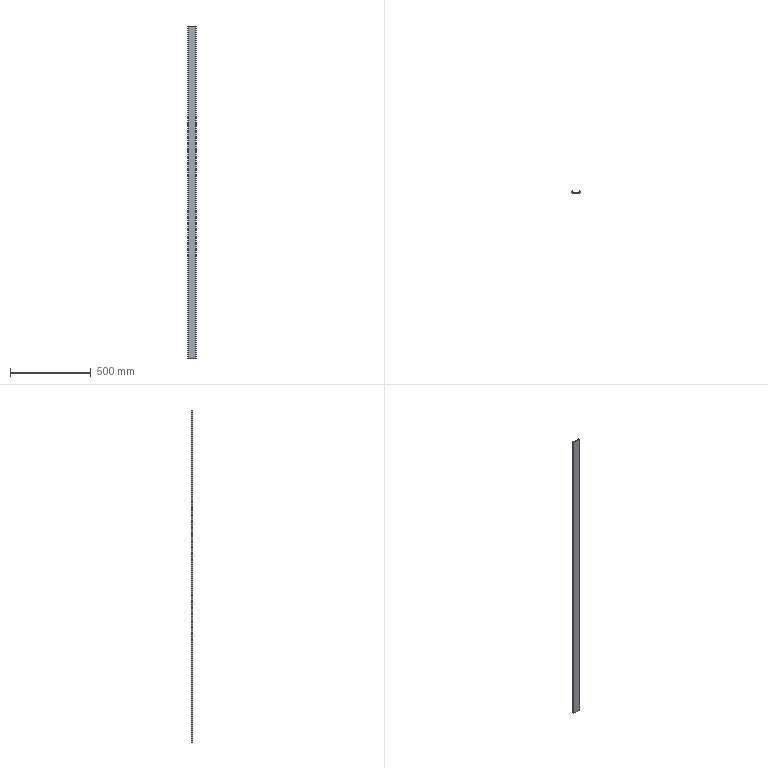Part | STEP file | 31E-01030QY25 | 1 solid | 32 faces | box 50 x 9.195 x 2050 mm | volume 179814 mm3 | cylinder 16 | plane 16 | commonest cylinder face diameters 1 x8 1.2 x6 2 x2
STEP:
#1=CARTESIAN_POINT('',(0.2485,8.595,1025.));
#2=VERTEX_POINT('',#1);
#3=CARTESIAN_POINT('',(0.4243,8.171,1025.));
#4=VERTEX_POINT('',#3);
#5=CARTESIAN_POINT('',(0.8485,8.595,1025.));
#6=DIRECTION('',(0.,0.,-1.));
#7=AXIS2_PLACEMENT_3D('',#5,#6,$);
#8=CIRCLE('',#7,0.6);
#9=EDGE_CURVE('',#2,#4,#8,.F.);
#10=ORIENTED_EDGE('',*,*,#9,.F.);
#11=CARTESIAN_POINT('',(0.2485,8.595,-1025.));
#12=VERTEX_POINT('',#11);
#13=CARTESIAN_POINT('',(0.2485,8.595,1025.));
#14=DIRECTION('',(0.,0.,-1.));
#15=VECTOR('',#14,1.);
#16=LINE('',#13,#15);
#17=EDGE_CURVE('',#2,#12,#16,.T.);
#18=ORIENTED_EDGE('',*,*,#17,.T.);
#19=CARTESIAN_POINT('',(0.4243,8.171,-1025.));
#20=VERTEX_POINT('',#19);
#21=CARTESIAN_POINT('',(0.8485,8.595,-1025.));
#22=DIRECTION('',(0.,0.,-1.));
#23=AXIS2_PLACEMENT_3D('',#21,#22,$);
#24=CIRCLE('',#23,0.6);
#25=EDGE_CURVE('',#20,#12,#24,.T.);
#26=ORIENTED_EDGE('',*,*,#25,.F.);
#27=CARTESIAN_POINT('',(0.4243,8.171,1025.));
#28=DIRECTION('',(0.,0.,-1.));
#29=VECTOR('',#28,1.);
#30=LINE('',#27,#29);
#31=EDGE_CURVE('',#4,#20,#30,.T.);
#32=ORIENTED_EDGE('',*,*,#31,.F.);
#33=EDGE_LOOP('',(#10,#18,#26,#32));
#34=FACE_OUTER_BOUND('',#33,.T.);
#35=CARTESIAN_POINT('',(0.8485,8.595,1025.));
#36=DIRECTION('',(0.,0.,-1.));
#37=DIRECTION('',(1.,0.,0.));
#38=AXIS2_PLACEMENT_3D('',#35,#36,#37);
#39=CYLINDRICAL_SURFACE('',#38,0.6);
#40=ADVANCED_FACE('',(#34),#39,.T.);
#41=CARTESIAN_POINT('',(1.273,9.019,1025.));
#42=VERTEX_POINT('',#41);
#43=CARTESIAN_POINT('',(0.4243,9.019,1025.));
#44=VERTEX_POINT('',#43);
#45=CARTESIAN_POINT('',(1.273,9.019,1025.));
#46=CARTESIAN_POINT('',(1.219,9.073,1025.));
#47=CARTESIAN_POINT('',(1.158,9.118,1025.));
#48=CARTESIAN_POINT('',(1.089,9.152,1025.));
#49=CARTESIAN_POINT('',(0.9442,9.199,1025.));
#50=CARTESIAN_POINT('',(0.7916,9.2,1025.));
#51=CARTESIAN_POINT('',(0.7159,9.188,1025.));
#52=CARTESIAN_POINT('',(0.6071,9.152,1025.));
#53=CARTESIAN_POINT('',(0.5104,9.093,1025.));
#54=CARTESIAN_POINT('',(0.4796,9.07,1025.));
#55=CARTESIAN_POINT('',(0.4509,9.046,1025.));
#56=CARTESIAN_POINT('',(0.4243,9.019,1025.));
#57=B_SPLINE_CURVE_WITH_KNOTS('',5,(#45,#46,#47,#48,#49,#50,#51,#52,#53,#54,#55,#56),.UNSPECIFIED.,.F.,.U.,(6,3,3,6),(0.,0.5331,1.066,1.332),.UNSPECIFIED.);
#58=EDGE_CURVE('',#42,#44,#57,.T.);
#59=ORIENTED_EDGE('',*,*,#58,.T.);
#60=CARTESIAN_POINT('',(0.4243,9.019,1025.));
#61=CARTESIAN_POINT('',(0.3843,8.979,1025.));
#62=CARTESIAN_POINT('',(0.349,8.935,1025.));
#63=CARTESIAN_POINT('',(0.3192,8.886,1025.));
#64=CARTESIAN_POINT('',(0.2795,8.8,1025.));
#65=CARTESIAN_POINT('',(0.2574,8.708,1025.));
#66=CARTESIAN_POINT('',(0.2515,8.67,1025.));
#67=CARTESIAN_POINT('',(0.2485,8.633,1025.));
#68=CARTESIAN_POINT('',(0.2485,8.595,1025.));
#69=B_SPLINE_CURVE_WITH_KNOTS('',5,(#60,#61,#62,#63,#64,#65,#66,#67,#68),.UNSPECIFIED.,.F.,.U.,(6,3,6),(0.,0.3999,0.6659),.UNSPECIFIED.);
#70=EDGE_CURVE('',#44,#2,#69,.T.);
#71=ORIENTED_EDGE('',*,*,#70,.T.);
#72=ORIENTED_EDGE('',*,*,#9,.T.);
#73=CARTESIAN_POINT('',(2.898,5.697,1025.));
#74=VERTEX_POINT('',#73);
#75=CARTESIAN_POINT('',(1.661,6.934,1025.));
#76=DIRECTION('',(0.7071,-0.7071,0.));
#77=VECTOR('',#76,1.);
#78=LINE('',#75,#77);
#79=EDGE_CURVE('',#4,#74,#78,.T.);
#80=ORIENTED_EDGE('',*,*,#79,.T.);
#81=CARTESIAN_POINT('',(0.3706,5.02,1025.));
#82=VERTEX_POINT('',#81);
#83=CARTESIAN_POINT('',(1.634,5.359,1025.));
#84=DIRECTION('',(-0.9659,-0.2588,0.));
#85=VECTOR('',#84,1.);
#86=LINE('',#83,#85);
#87=EDGE_CURVE('',#74,#82,#86,.T.);
#88=ORIENTED_EDGE('',*,*,#87,.T.);
#89=CARTESIAN_POINT('',(0.,4.537,1025.));
#90=VERTEX_POINT('',#89);
#91=CARTESIAN_POINT('',(0.3706,5.02,1025.));
#92=CARTESIAN_POINT('',(0.32,5.007,1025.));
#93=CARTESIAN_POINT('',(0.2712,4.986,1025.));
#94=CARTESIAN_POINT('',(0.2253,4.96,1025.));
#95=CARTESIAN_POINT('',(0.1416,4.896,1025.));
#96=CARTESIAN_POINT('',(0.07725,4.812,1025.));
#97=CARTESIAN_POINT('',(0.05076,4.766,1025.));
#98=CARTESIAN_POINT('',(0.02052,4.693,1025.));
#99=CARTESIAN_POINT('',(0.005155,4.616,1025.));
#100=CARTESIAN_POINT('',(0.001709,4.589,1025.));
#101=CARTESIAN_POINT('',(0.,4.563,1025.));
#102=CARTESIAN_POINT('',(0.,4.537,1025.));
#103=B_SPLINE_CURVE_WITH_KNOTS('',5,(#91,#92,#93,#94,#95,#96,#97,#98,#99,#100,#101,#102),.UNSPECIFIED.,.F.,.U.,(6,3,3,6),(0.,0.3702,0.7405,0.9253),.UNSPECIFIED.);
#104=EDGE_CURVE('',#82,#90,#103,.T.);
#105=ORIENTED_EDGE('',*,*,#104,.T.);
#106=CARTESIAN_POINT('',(0.,1.,1025.));
#107=VERTEX_POINT('',#106);
#108=CARTESIAN_POINT('',(0.,2.769,1025.));
#109=DIRECTION('',(0.,-1.,0.));
#110=VECTOR('',#109,1.);
#111=LINE('',#108,#110);
#112=EDGE_CURVE('',#90,#107,#111,.T.);
#113=ORIENTED_EDGE('',*,*,#112,.T.);
#114=CARTESIAN_POINT('',(1.,0.,1025.));
#115=VERTEX_POINT('',#114);
#116=CARTESIAN_POINT('',(0.,1.,1025.));
#117=CARTESIAN_POINT('',(0.,0.902,1025.));
#118=CARTESIAN_POINT('',(0.012,0.804,1025.));
#119=CARTESIAN_POINT('',(0.036,0.708,1025.));
#120=CARTESIAN_POINT('',(0.107,0.5238,1025.));
#121=CARTESIAN_POINT('',(0.2204,0.3622,1025.));
#122=CARTESIAN_POINT('',(0.2868,0.2888,1025.));
#123=CARTESIAN_POINT('',(0.4361,0.1597,1025.));
#124=CARTESIAN_POINT('',(0.6122,0.0704,1025.));
#125=CARTESIAN_POINT('',(0.7053,0.03682,1025.));
#126=CARTESIAN_POINT('',(0.8215,0.01049,1025.));
#127=CARTESIAN_POINT('',(0.9393,0.001534,1025.));
#128=CARTESIAN_POINT('',(0.9596,0.0005109,1025.));
#129=CARTESIAN_POINT('',(0.9798,0.000000001,1025.));
#130=CARTESIAN_POINT('',(1.,0.000000001,1025.));
#131=B_SPLINE_CURVE_WITH_KNOTS('',5,(#116,#117,#118,#119,#120,#121,#122,#123,#124,#125,#126,#127,#128,#129,#130),.UNSPECIFIED.,.F.,.U.,(6,3,3,3,6),(0.,0.6928,1.386,2.078,2.221),.UNSPECIFIED.);
#132=EDGE_CURVE('',#107,#115,#131,.T.);
#133=ORIENTED_EDGE('',*,*,#132,.T.);
#134=CARTESIAN_POINT('',(49.,0.,1025.));
#135=VERTEX_POINT('',#134);
#136=CARTESIAN_POINT('',(25.,0.000000001,1025.));
#137=DIRECTION('',(1.,0.,0.));
#138=VECTOR('',#137,1.);
#139=LINE('',#136,#138);
#140=EDGE_CURVE('',#115,#135,#139,.T.);
#141=ORIENTED_EDGE('',*,*,#140,.T.);
#142=CARTESIAN_POINT('',(50.,1.,1025.));
#143=VERTEX_POINT('',#142);
#144=CARTESIAN_POINT('',(49.,0.000000001,1025.));
#145=CARTESIAN_POINT('',(49.098,0.000000001,1025.));
#146=CARTESIAN_POINT('',(49.196,0.012,1025.));
#147=CARTESIAN_POINT('',(49.292,0.036,1025.));
#148=CARTESIAN_POINT('',(49.476,0.107,1025.));
#149=CARTESIAN_POINT('',(49.638,0.2204,1025.));
#150=CARTESIAN_POINT('',(49.711,0.2868,1025.));
#151=CARTESIAN_POINT('',(49.84,0.4361,1025.));
#152=CARTESIAN_POINT('',(49.93,0.6122,1025.));
#153=CARTESIAN_POINT('',(49.963,0.7053,1025.));
#154=CARTESIAN_POINT('',(49.99,0.8215,1025.));
#155=CARTESIAN_POINT('',(49.998,0.9393,1025.));
#156=CARTESIAN_POINT('',(49.999,0.9596,1025.));
#157=CARTESIAN_POINT('',(50.,0.9798,1025.));
#158=CARTESIAN_POINT('',(50.,1.,1025.));
#159=B_SPLINE_CURVE_WITH_KNOTS('',5,(#144,#145,#146,#147,#148,#149,#150,#151,#152,#153,#154,#155,#156,#157,#158),.UNSPECIFIED.,.F.,.U.,(6,3,3,3,6),(0.,0.6928,1.386,2.078,2.221),.UNSPECIFIED.);
#160=EDGE_CURVE('',#135,#143,#159,.T.);
#161=ORIENTED_EDGE('',*,*,#160,.T.);
#162=CARTESIAN_POINT('',(50.,4.537,1025.));
#163=VERTEX_POINT('',#162);
#164=CARTESIAN_POINT('',(50.,2.769,1025.));
#165=DIRECTION('',(0.,1.,0.));
#166=VECTOR('',#165,1.);
#167=LINE('',#164,#166);
#168=EDGE_CURVE('',#143,#163,#167,.T.);
#169=ORIENTED_EDGE('',*,*,#168,.T.);
#170=CARTESIAN_POINT('',(49.629,5.02,1025.));
#171=VERTEX_POINT('',#170);
#172=CARTESIAN_POINT('',(50.,4.537,1025.));
#173=CARTESIAN_POINT('',(50.,4.589,1025.));
#174=CARTESIAN_POINT('',(49.993,4.642,1025.));
#175=CARTESIAN_POINT('',(49.979,4.693,1025.));
#176=CARTESIAN_POINT('',(49.939,4.791,1025.));
#177=CARTESIAN_POINT('',(49.875,4.874,1025.));
#178=CARTESIAN_POINT('',(49.837,4.912,1025.));
#179=CARTESIAN_POINT('',(49.774,4.96,1025.));
#180=CARTESIAN_POINT('',(49.704,4.995,1025.));
#181=CARTESIAN_POINT('',(49.679,5.005,1025.));
#182=CARTESIAN_POINT('',(49.655,5.013,1025.));
#183=CARTESIAN_POINT('',(49.629,5.02,1025.));
#184=B_SPLINE_CURVE_WITH_KNOTS('',5,(#172,#173,#174,#175,#176,#177,#178,#179,#180,#181,#182,#183),.UNSPECIFIED.,.F.,.U.,(6,3,3,6),(0.,0.3702,0.7405,0.9253),.UNSPECIFIED.);
#185=EDGE_CURVE('',#163,#171,#184,.T.);
#186=ORIENTED_EDGE('',*,*,#185,.T.);
#187=CARTESIAN_POINT('',(47.102,5.697,1025.));
#188=VERTEX_POINT('',#187);
#189=CARTESIAN_POINT('',(48.366,5.359,1025.));
#190=DIRECTION('',(-0.9659,0.2588,0.));
#191=VECTOR('',#190,1.);
#192=LINE('',#189,#191);
#193=EDGE_CURVE('',#171,#188,#192,.T.);
#194=ORIENTED_EDGE('',*,*,#193,.T.);
#195=CARTESIAN_POINT('',(49.576,8.171,1025.));
#196=VERTEX_POINT('',#195);
#197=CARTESIAN_POINT('',(48.339,6.934,1025.));
#198=DIRECTION('',(0.7071,0.7071,0.));
#199=VECTOR('',#198,1.);
#200=LINE('',#197,#199);
#201=EDGE_CURVE('',#188,#196,#200,.T.);
#202=ORIENTED_EDGE('',*,*,#201,.T.);
#203=CARTESIAN_POINT('',(49.751,8.595,1025.));
#204=VERTEX_POINT('',#203);
#205=CARTESIAN_POINT('',(49.576,8.171,1025.));
#206=CARTESIAN_POINT('',(49.629,8.224,1025.));
#207=CARTESIAN_POINT('',(49.674,8.286,1025.));
#208=CARTESIAN_POINT('',(49.709,8.354,1025.));
#209=CARTESIAN_POINT('',(49.738,8.445,1025.));
#210=CARTESIAN_POINT('',(49.749,8.539,1025.));
#211=CARTESIAN_POINT('',(49.751,8.557,1025.));
#212=CARTESIAN_POINT('',(49.751,8.576,1025.));
#213=CARTESIAN_POINT('',(49.751,8.595,1025.));
#214=B_SPLINE_CURVE_WITH_KNOTS('',5,(#205,#206,#207,#208,#209,#210,#211,#212,#213),.UNSPECIFIED.,.F.,.U.,(6,3,6),(0.,0.5331,0.6664),.UNSPECIFIED.);
#215=EDGE_CURVE('',#196,#204,#214,.T.);
#216=ORIENTED_EDGE('',*,*,#215,.T.);
#217=CARTESIAN_POINT('',(49.576,9.019,1025.));
#218=VERTEX_POINT('',#217);
#219=CARTESIAN_POINT('',(49.751,8.595,1025.));
#220=CARTESIAN_POINT('',(49.751,8.652,1025.));
#221=CARTESIAN_POINT('',(49.745,8.708,1025.));
#222=CARTESIAN_POINT('',(49.731,8.764,1025.));
#223=CARTESIAN_POINT('',(49.699,8.853,1025.));
#224=CARTESIAN_POINT('',(49.649,8.933,1025.));
#225=CARTESIAN_POINT('',(49.627,8.964,1025.));
#226=CARTESIAN_POINT('',(49.602,8.993,1025.));
#227=CARTESIAN_POINT('',(49.576,9.019,1025.));
#228=B_SPLINE_CURVE_WITH_KNOTS('',5,(#219,#220,#221,#222,#223,#224,#225,#226,#227),.UNSPECIFIED.,.F.,.U.,(6,3,6),(0.6664,1.066,1.332),.UNSPECIFIED.);
#229=EDGE_CURVE('',#204,#218,#228,.T.);
#230=ORIENTED_EDGE('',*,*,#229,.T.);
#231=CARTESIAN_POINT('',(48.727,9.019,1025.));
#232=VERTEX_POINT('',#231);
#233=CARTESIAN_POINT('',(49.576,9.019,1025.));
#234=CARTESIAN_POINT('',(49.522,9.073,1025.));
#235=CARTESIAN_POINT('',(49.461,9.118,1025.));
#236=CARTESIAN_POINT('',(49.392,9.152,1025.));
#237=CARTESIAN_POINT('',(49.247,9.199,1025.));
#238=CARTESIAN_POINT('',(49.095,9.2,1025.));
#239=CARTESIAN_POINT('',(49.019,9.188,1025.));
#240=CARTESIAN_POINT('',(48.91,9.152,1025.));
#241=CARTESIAN_POINT('',(48.813,9.093,1025.));
#242=CARTESIAN_POINT('',(48.782,9.07,1025.));
#243=CARTESIAN_POINT('',(48.754,9.046,1025.));
#244=CARTESIAN_POINT('',(48.727,9.019,1025.));
#245=B_SPLINE_CURVE_WITH_KNOTS('',5,(#233,#234,#235,#236,#237,#238,#239,#240,#241,#242,#243,#244),.UNSPECIFIED.,.F.,.U.,(6,3,3,6),(0.,0.5331,1.066,1.332),.UNSPECIFIED.);
#246=EDGE_CURVE('',#218,#232,#245,.T.);
#247=ORIENTED_EDGE('',*,*,#246,.T.);
#248=CARTESIAN_POINT('',(45.396,5.688,1025.));
#249=VERTEX_POINT('',#248);
#250=CARTESIAN_POINT('',(47.062,7.354,1025.));
#251=DIRECTION('',(-0.7071,-0.7071,0.));
#252=VECTOR('',#251,1.);
#253=LINE('',#250,#252);
#254=EDGE_CURVE('',#232,#249,#253,.T.);
#255=ORIENTED_EDGE('',*,*,#254,.T.);
#256=CARTESIAN_POINT('',(45.25,5.335,1025.));
#257=VERTEX_POINT('',#256);
#258=CARTESIAN_POINT('',(45.396,5.688,1025.));
#259=CARTESIAN_POINT('',(45.363,5.655,1025.));
#260=CARTESIAN_POINT('',(45.334,5.618,1025.));
#261=CARTESIAN_POINT('',(45.309,5.577,1025.));
#262=CARTESIAN_POINT('',(45.276,5.506,1025.));
#263=CARTESIAN_POINT('',(45.257,5.429,1025.));
#264=CARTESIAN_POINT('',(45.252,5.398,1025.));
#265=CARTESIAN_POINT('',(45.25,5.366,1025.));
#266=CARTESIAN_POINT('',(45.25,5.335,1025.));
#267=B_SPLINE_CURVE_WITH_KNOTS('',5,(#258,#259,#260,#261,#262,#263,#264,#265,#266),.UNSPECIFIED.,.F.,.U.,(6,3,6),(0.,0.3332,0.5549),.UNSPECIFIED.);
#268=EDGE_CURVE('',#249,#257,#267,.T.);
#269=ORIENTED_EDGE('',*,*,#268,.T.);
#270=CARTESIAN_POINT('',(45.621,4.852,1025.));
#271=VERTEX_POINT('',#270);
#272=CARTESIAN_POINT('',(45.25,5.335,1025.));
#273=CARTESIAN_POINT('',(45.25,5.283,1025.));
#274=CARTESIAN_POINT('',(45.257,5.23,1025.));
#275=CARTESIAN_POINT('',(45.27,5.179,1025.));
#276=CARTESIAN_POINT('',(45.311,5.081,1025.));
#277=CARTESIAN_POINT('',(45.375,4.998,1025.));
#278=CARTESIAN_POINT('',(45.413,4.96,1025.));
#279=CARTESIAN_POINT('',(45.476,4.912,1025.));
#280=CARTESIAN_POINT('',(45.546,4.877,1025.));
#281=CARTESIAN_POINT('',(45.57,4.867,1025.));
#282=CARTESIAN_POINT('',(45.595,4.859,1025.));
#283=CARTESIAN_POINT('',(45.621,4.852,1025.));
#284=B_SPLINE_CURVE_WITH_KNOTS('',5,(#272,#273,#274,#275,#276,#277,#278,#279,#280,#281,#282,#283),.UNSPECIFIED.,.F.,.U.,(6,3,3,6),(0.,0.3702,0.7405,0.9253),.UNSPECIFIED.);
#285=EDGE_CURVE('',#257,#271,#284,.T.);
#286=ORIENTED_EDGE('',*,*,#285,.T.);
#287=CARTESIAN_POINT('',(48.8,4.,1025.));
#288=VERTEX_POINT('',#287);
#289=CARTESIAN_POINT('',(47.21,4.426,1025.));
#290=DIRECTION('',(0.9659,-0.2588,0.));
#291=VECTOR('',#290,1.);
#292=LINE('',#289,#291);
#293=EDGE_CURVE('',#271,#288,#292,.T.);
#294=ORIENTED_EDGE('',*,*,#293,.T.);
#295=CARTESIAN_POINT('',(48.8,1.7,1025.));
#296=VERTEX_POINT('',#295);
#297=CARTESIAN_POINT('',(48.8,2.85,1025.));
#298=DIRECTION('',(0.,-1.,0.));
#299=VECTOR('',#298,1.);
#300=LINE('',#297,#299);
#301=EDGE_CURVE('',#288,#296,#300,.T.);
#302=ORIENTED_EDGE('',*,*,#301,.T.);
#303=CARTESIAN_POINT('',(48.3,1.2,1025.));
#304=VERTEX_POINT('',#303);
#305=CARTESIAN_POINT('',(48.3,1.7,1025.));
#306=DIRECTION('',(0.,0.,-1.));
#307=AXIS2_PLACEMENT_3D('',#305,#306,$);
#308=CIRCLE('',#307,0.5);
#309=EDGE_CURVE('',#296,#304,#308,.T.);
#310=ORIENTED_EDGE('',*,*,#309,.T.);
#311=CARTESIAN_POINT('',(1.7,1.2,1025.));
#312=VERTEX_POINT('',#311);
#313=CARTESIAN_POINT('',(25.,1.2,1025.));
#314=DIRECTION('',(-1.,0.,0.));
#315=VECTOR('',#314,1.);
#316=LINE('',#313,#315);
#317=EDGE_CURVE('',#304,#312,#316,.T.);
#318=ORIENTED_EDGE('',*,*,#317,.T.);
#319=CARTESIAN_POINT('',(1.2,1.7,1025.));
#320=VERTEX_POINT('',#319);
#321=CARTESIAN_POINT('',(1.7,1.7,1025.));
#322=DIRECTION('',(0.,0.,-1.));
#323=AXIS2_PLACEMENT_3D('',#321,#322,$);
#324=CIRCLE('',#323,0.5);
#325=EDGE_CURVE('',#312,#320,#324,.T.);
#326=ORIENTED_EDGE('',*,*,#325,.T.);
#327=CARTESIAN_POINT('',(1.2,4.,1025.));
#328=VERTEX_POINT('',#327);
#329=CARTESIAN_POINT('',(1.2,2.85,1025.));
#330=DIRECTION('',(0.,1.,0.));
#331=VECTOR('',#330,1.);
#332=LINE('',#329,#331);
#333=EDGE_CURVE('',#320,#328,#332,.T.);
#334=ORIENTED_EDGE('',*,*,#333,.T.);
#335=CARTESIAN_POINT('',(4.379,4.852,1025.));
#336=VERTEX_POINT('',#335);
#337=CARTESIAN_POINT('',(2.79,4.426,1025.));
#338=DIRECTION('',(0.9659,0.2588,0.));
#339=VECTOR('',#338,1.);
#340=LINE('',#337,#339);
#341=EDGE_CURVE('',#328,#336,#340,.T.);
#342=ORIENTED_EDGE('',*,*,#341,.T.);
#343=CARTESIAN_POINT('',(4.75,5.335,1025.));
#344=VERTEX_POINT('',#343);
#345=CARTESIAN_POINT('',(4.379,4.852,1025.));
#346=CARTESIAN_POINT('',(4.446,4.87,1025.));
#347=CARTESIAN_POINT('',(4.51,4.899,1025.));
#348=CARTESIAN_POINT('',(4.568,4.94,1025.));
#349=CARTESIAN_POINT('',(4.662,5.034,1025.));
#350=CARTESIAN_POINT('',(4.722,5.152,1025.));
#351=CARTESIAN_POINT('',(4.741,5.212,1025.));
#352=CARTESIAN_POINT('',(4.75,5.273,1025.));
#353=CARTESIAN_POINT('',(4.75,5.335,1025.));
#354=B_SPLINE_CURVE_WITH_KNOTS('',5,(#345,#346,#347,#348,#349,#350,#351,#352,#353),.UNSPECIFIED.,.F.,.U.,(6,3,6),(0.,0.4899,0.9256),.UNSPECIFIED.);
#355=EDGE_CURVE('',#336,#344,#354,.T.);
#356=ORIENTED_EDGE('',*,*,#355,.T.);
#357=CARTESIAN_POINT('',(4.604,5.688,1025.));
#358=VERTEX_POINT('',#357);
#359=CARTESIAN_POINT('',(4.75,5.335,1025.));
#360=CARTESIAN_POINT('',(4.75,5.343,1025.));
#361=CARTESIAN_POINT('',(4.75,5.35,1025.));
#362=CARTESIAN_POINT('',(4.75,5.358,1025.));
#363=CARTESIAN_POINT('',(4.745,5.435,1025.));
#364=CARTESIAN_POINT('',(4.726,5.51,1025.));
#365=CARTESIAN_POINT('',(4.697,5.575,1025.));
#366=CARTESIAN_POINT('',(4.657,5.634,1025.));
#367=CARTESIAN_POINT('',(4.607,5.685,1025.));
#368=CARTESIAN_POINT('',(4.606,5.686,1025.));
#369=CARTESIAN_POINT('',(4.605,5.687,1025.));
#370=CARTESIAN_POINT('',(4.604,5.688,1025.));
#371=B_SPLINE_CURVE_WITH_KNOTS('',5,(#359,#360,#361,#362,#363,#364,#365,#366,#367,#368,#369,#370),.UNSPECIFIED.,.F.,.U.,(6,3,3,6),(0.9256,0.9798,1.47,1.481),.UNSPECIFIED.);
#372=EDGE_CURVE('',#344,#358,#371,.T.);
#373=ORIENTED_EDGE('',*,*,#372,.T.);
#374=CARTESIAN_POINT('',(2.938,7.354,1025.));
#375=DIRECTION('',(-0.7071,0.7071,0.));
#376=VECTOR('',#375,1.);
#377=LINE('',#374,#376);
#378=EDGE_CURVE('',#358,#42,#377,.T.);
#379=ORIENTED_EDGE('',*,*,#378,.T.);
#380=EDGE_LOOP('',(#59,#71,#72,#80,#88,#105,#113,#133,#141,#161,#169,#186,#194,#202,#216,#230,#247,#255,#269,#286,#294,#302,#310,#318,#326,#334,#342,#356,#373,#379));
#381=FACE_OUTER_BOUND('',#380,.T.);
#382=CARTESIAN_POINT('',(0.,1.2,1025.));
#383=DIRECTION('',(0.,0.,-1.));
#384=DIRECTION('',(-1.,0.,0.));
#385=AXIS2_PLACEMENT_3D('',#382,#383,#384);
#386=PLANE('',#385);
#387=ADVANCED_FACE('',(#381),#386,.F.);
#388=ORIENTED_EDGE('',*,*,#17,.F.);
#389=ORIENTED_EDGE('',*,*,#70,.F.);
#390=CARTESIAN_POINT('',(0.4243,9.019,-1025.));
#391=VERTEX_POINT('',#390);
#392=CARTESIAN_POINT('',(0.4243,9.019,1025.));
#393=DIRECTION('',(0.,0.,-1.));
#394=VECTOR('',#393,1.);
#395=LINE('',#392,#394);
#396=EDGE_CURVE('',#44,#391,#395,.T.);
#397=ORIENTED_EDGE('',*,*,#396,.T.);
#398=CARTESIAN_POINT('',(0.8485,8.595,-1025.));
#399=DIRECTION('',(0.,0.,-1.));
#400=AXIS2_PLACEMENT_3D('',#398,#399,$);
#401=CIRCLE('',#400,0.6);
#402=EDGE_CURVE('',#12,#391,#401,.T.);
#403=ORIENTED_EDGE('',*,*,#402,.F.);
#404=EDGE_LOOP('',(#388,#389,#397,#403));
#405=FACE_OUTER_BOUND('',#404,.T.);
#406=CARTESIAN_POINT('',(0.8485,8.595,1025.));
#407=DIRECTION('',(0.,0.,-1.));
#408=DIRECTION('',(-1.,0.,0.));
#409=AXIS2_PLACEMENT_3D('',#406,#407,#408);
#410=CYLINDRICAL_SURFACE('',#409,0.6);
#411=ADVANCED_FACE('',(#405),#410,.T.);
#412=CARTESIAN_POINT('',(2.898,5.697,-1025.));
#413=VERTEX_POINT('',#412);
#414=CARTESIAN_POINT('',(1.661,6.934,-1025.));
#415=DIRECTION('',(0.7071,-0.7071,0.));
#416=VECTOR('',#415,1.);
#417=LINE('',#414,#416);
#418=EDGE_CURVE('',#20,#413,#417,.T.);
#419=ORIENTED_EDGE('',*,*,#418,.F.);
#420=ORIENTED_EDGE('',*,*,#25,.T.);
#421=ORIENTED_EDGE('',*,*,#402,.T.);
#422=CARTESIAN_POINT('',(1.273,9.019,-1025.));
#423=VERTEX_POINT('',#422);
#424=CARTESIAN_POINT('',(0.8485,8.595,-1025.));
#425=DIRECTION('',(0.,0.,-1.));
#426=AXIS2_PLACEMENT_3D('',#424,#425,$);
#427=CIRCLE('',#426,0.6);
#428=EDGE_CURVE('',#391,#423,#427,.T.);
#429=ORIENTED_EDGE('',*,*,#428,.T.);
#430=CARTESIAN_POINT('',(4.604,5.688,-1025.));
#431=VERTEX_POINT('',#430);
#432=CARTESIAN_POINT('',(2.938,7.354,-1025.));
#433=DIRECTION('',(-0.7071,0.7071,0.));
#434=VECTOR('',#433,1.);
#435=LINE('',#432,#434);
#436=EDGE_CURVE('',#431,#423,#435,.T.);
#437=ORIENTED_EDGE('',*,*,#436,.F.);
#438=CARTESIAN_POINT('',(4.75,5.335,-1025.));
#439=VERTEX_POINT('',#438);
#440=CARTESIAN_POINT('',(4.25,5.335,-1025.));
#441=DIRECTION('',(0.,0.,-1.));
#442=AXIS2_PLACEMENT_3D('',#440,#441,$);
#443=CIRCLE('',#442,0.5);
#444=EDGE_CURVE('',#431,#439,#443,.T.);
#445=ORIENTED_EDGE('',*,*,#444,.T.);
#446=CARTESIAN_POINT('',(4.379,4.852,-1025.));
#447=VERTEX_POINT('',#446);
#448=CARTESIAN_POINT('',(4.25,5.335,-1025.));
#449=DIRECTION('',(0.,0.,-1.));
#450=AXIS2_PLACEMENT_3D('',#448,#449,$);
#451=CIRCLE('',#450,0.5);
#452=EDGE_CURVE('',#439,#447,#451,.T.);
#453=ORIENTED_EDGE('',*,*,#452,.T.);
#454=CARTESIAN_POINT('',(1.2,4.,-1025.));
#455=VERTEX_POINT('',#454);
#456=CARTESIAN_POINT('',(2.79,4.426,-1025.));
#457=DIRECTION('',(0.9659,0.2588,0.));
#458=VECTOR('',#457,1.);
#459=LINE('',#456,#458);
#460=EDGE_CURVE('',#455,#447,#459,.T.);
#461=ORIENTED_EDGE('',*,*,#460,.F.);
#462=CARTESIAN_POINT('',(1.2,1.7,-1025.));
#463=VERTEX_POINT('',#462);
#464=CARTESIAN_POINT('',(1.2,2.85,-1025.));
#465=DIRECTION('',(0.,1.,0.));
#466=VECTOR('',#465,1.);
#467=LINE('',#464,#466);
#468=EDGE_CURVE('',#463,#455,#467,.T.);
#469=ORIENTED_EDGE('',*,*,#468,.F.);
#470=CARTESIAN_POINT('',(1.7,1.2,-1025.));
#471=VERTEX_POINT('',#470);
#472=CARTESIAN_POINT('',(1.2,1.7,-1025.));
#473=CARTESIAN_POINT('',(1.2,1.637,-1025.));
#474=CARTESIAN_POINT('',(1.21,1.574,-1025.));
#475=CARTESIAN_POINT('',(1.23,1.514,-1025.));
#476=CARTESIAN_POINT('',(1.288,1.4,-1025.));
#477=CARTESIAN_POINT('',(1.377,1.31,-1025.));
#478=CARTESIAN_POINT('',(1.429,1.273,-1025.));
#479=CARTESIAN_POINT('',(1.514,1.23,-1025.));
#480=CARTESIAN_POINT('',(1.606,1.207,-1025.));
#481=CARTESIAN_POINT('',(1.637,1.202,-1025.));
#482=CARTESIAN_POINT('',(1.669,1.2,-1025.));
#483=CARTESIAN_POINT('',(1.7,1.2,-1025.));
#484=B_SPLINE_CURVE_WITH_KNOTS('',5,(#472,#473,#474,#475,#476,#477,#478,#479,#480,#481,#482,#483),.UNSPECIFIED.,.F.,.U.,(6,3,3,6),(0.,0.4443,0.8886,1.11),.UNSPECIFIED.);
#485=EDGE_CURVE('',#463,#471,#484,.T.);
#486=ORIENTED_EDGE('',*,*,#485,.T.);
#487=CARTESIAN_POINT('',(48.3,1.2,-1025.));
#488=VERTEX_POINT('',#487);
#489=CARTESIAN_POINT('',(25.,1.2,-1025.));
#490=DIRECTION('',(-1.,0.,0.));
#491=VECTOR('',#490,1.);
#492=LINE('',#489,#491);
#493=EDGE_CURVE('',#488,#471,#492,.T.);
#494=ORIENTED_EDGE('',*,*,#493,.F.);
#495=CARTESIAN_POINT('',(48.8,1.7,-1025.));
#496=VERTEX_POINT('',#495);
#497=CARTESIAN_POINT('',(48.3,1.2,-1025.));
#498=CARTESIAN_POINT('',(48.363,1.2,-1025.));
#499=CARTESIAN_POINT('',(48.426,1.21,-1025.));
#500=CARTESIAN_POINT('',(48.486,1.23,-1025.));
#501=CARTESIAN_POINT('',(48.6,1.288,-1025.));
#502=CARTESIAN_POINT('',(48.69,1.377,-1025.));
#503=CARTESIAN_POINT('',(48.727,1.429,-1025.));
#504=CARTESIAN_POINT('',(48.77,1.514,-1025.));
#505=CARTESIAN_POINT('',(48.793,1.606,-1025.));
#506=CARTESIAN_POINT('',(48.798,1.637,-1025.));
#507=CARTESIAN_POINT('',(48.8,1.669,-1025.));
#508=CARTESIAN_POINT('',(48.8,1.7,-1025.));
#509=B_SPLINE_CURVE_WITH_KNOTS('',5,(#497,#498,#499,#500,#501,#502,#503,#504,#505,#506,#507,#508),.UNSPECIFIED.,.F.,.U.,(6,3,3,6),(0.,0.4443,0.8886,1.11),.UNSPECIFIED.);
#510=EDGE_CURVE('',#488,#496,#509,.T.);
#511=ORIENTED_EDGE('',*,*,#510,.T.);
#512=CARTESIAN_POINT('',(48.8,4.,-1025.));
#513=VERTEX_POINT('',#512);
#514=CARTESIAN_POINT('',(48.8,2.85,-1025.));
#515=DIRECTION('',(0.,-1.,0.));
#516=VECTOR('',#515,1.);
#517=LINE('',#514,#516);
#518=EDGE_CURVE('',#513,#496,#517,.T.);
#519=ORIENTED_EDGE('',*,*,#518,.F.);
#520=CARTESIAN_POINT('',(45.621,4.852,-1025.));
#521=VERTEX_POINT('',#520);
#522=CARTESIAN_POINT('',(47.21,4.426,-1025.));
#523=DIRECTION('',(0.9659,-0.2588,0.));
#524=VECTOR('',#523,1.);
#525=LINE('',#522,#524);
#526=EDGE_CURVE('',#521,#513,#525,.T.);
#527=ORIENTED_EDGE('',*,*,#526,.F.);
#528=CARTESIAN_POINT('',(45.25,5.335,-1025.));
#529=VERTEX_POINT('',#528);
#530=CARTESIAN_POINT('',(45.75,5.335,-1025.));
#531=DIRECTION('',(0.,0.,-1.));
#532=AXIS2_PLACEMENT_3D('',#530,#531,$);
#533=CIRCLE('',#532,0.5);
#534=EDGE_CURVE('',#521,#529,#533,.T.);
#535=ORIENTED_EDGE('',*,*,#534,.T.);
#536=CARTESIAN_POINT('',(45.396,5.688,-1025.));
#537=VERTEX_POINT('',#536);
#538=CARTESIAN_POINT('',(45.75,5.335,-1025.));
#539=DIRECTION('',(0.,0.,-1.));
#540=AXIS2_PLACEMENT_3D('',#538,#539,$);
#541=CIRCLE('',#540,0.5);
#542=EDGE_CURVE('',#529,#537,#541,.T.);
#543=ORIENTED_EDGE('',*,*,#542,.T.);
#544=CARTESIAN_POINT('',(48.727,9.019,-1025.));
#545=VERTEX_POINT('',#544);
#546=CARTESIAN_POINT('',(47.062,7.354,-1025.));
#547=DIRECTION('',(-0.7071,-0.7071,0.));
#548=VECTOR('',#547,1.);
#549=LINE('',#546,#548);
#550=EDGE_CURVE('',#545,#537,#549,.T.);
#551=ORIENTED_EDGE('',*,*,#550,.F.);
#552=CARTESIAN_POINT('',(49.576,9.019,-1025.));
#553=VERTEX_POINT('',#552);
#554=CARTESIAN_POINT('',(49.151,8.595,-1025.));
#555=DIRECTION('',(0.,0.,-1.));
#556=AXIS2_PLACEMENT_3D('',#554,#555,$);
#557=CIRCLE('',#556,0.6);
#558=EDGE_CURVE('',#545,#553,#557,.T.);
#559=ORIENTED_EDGE('',*,*,#558,.T.);
#560=CARTESIAN_POINT('',(49.751,8.595,-1025.));
#561=VERTEX_POINT('',#560);
#562=CARTESIAN_POINT('',(49.151,8.595,-1025.));
#563=DIRECTION('',(0.,0.,-1.));
#564=AXIS2_PLACEMENT_3D('',#562,#563,$);
#565=CIRCLE('',#564,0.6);
#566=EDGE_CURVE('',#553,#561,#565,.T.);
#567=ORIENTED_EDGE('',*,*,#566,.T.);
#568=CARTESIAN_POINT('',(49.576,8.171,-1025.));
#569=VERTEX_POINT('',#568);
#570=CARTESIAN_POINT('',(49.151,8.595,-1025.));
#571=DIRECTION('',(0.,0.,-1.));
#572=AXIS2_PLACEMENT_3D('',#570,#571,$);
#573=CIRCLE('',#572,0.6);
#574=EDGE_CURVE('',#561,#569,#573,.T.);
#575=ORIENTED_EDGE('',*,*,#574,.T.);
#576=CARTESIAN_POINT('',(47.102,5.697,-1025.));
#577=VERTEX_POINT('',#576);
#578=CARTESIAN_POINT('',(48.339,6.934,-1025.));
#579=DIRECTION('',(0.7071,0.7071,0.));
#580=VECTOR('',#579,1.);
#581=LINE('',#578,#580);
#582=EDGE_CURVE('',#577,#569,#581,.T.);
#583=ORIENTED_EDGE('',*,*,#582,.F.);
#584=CARTESIAN_POINT('',(49.629,5.02,-1025.));
#585=VERTEX_POINT('',#584);
#586=CARTESIAN_POINT('',(48.366,5.359,-1025.));
#587=DIRECTION('',(-0.9659,0.2588,0.));
#588=VECTOR('',#587,1.);
#589=LINE('',#586,#588);
#590=EDGE_CURVE('',#585,#577,#589,.T.);
#591=ORIENTED_EDGE('',*,*,#590,.F.);
#592=CARTESIAN_POINT('',(50.,4.537,-1025.));
#593=VERTEX_POINT('',#592);
#594=CARTESIAN_POINT('',(49.5,4.537,-1025.));
#595=DIRECTION('',(0.,0.,-1.));
#596=AXIS2_PLACEMENT_3D('',#594,#595,$);
#597=CIRCLE('',#596,0.5);
#598=EDGE_CURVE('',#585,#593,#597,.T.);
#599=ORIENTED_EDGE('',*,*,#598,.T.);
#600=CARTESIAN_POINT('',(50.,1.,-1025.));
#601=VERTEX_POINT('',#600);
#602=CARTESIAN_POINT('',(50.,2.769,-1025.));
#603=DIRECTION('',(0.,1.,0.));
#604=VECTOR('',#603,1.);
#605=LINE('',#602,#604);
#606=EDGE_CURVE('',#601,#593,#605,.T.);
#607=ORIENTED_EDGE('',*,*,#606,.F.);
#608=CARTESIAN_POINT('',(49.,0.,-1025.));
#609=VERTEX_POINT('',#608);
#610=CARTESIAN_POINT('',(49.,1.,-1025.));
#611=DIRECTION('',(0.,0.,-1.));
#612=AXIS2_PLACEMENT_3D('',#610,#611,$);
#613=CIRCLE('',#612,1.);
#614=EDGE_CURVE('',#601,#609,#613,.T.);
#615=ORIENTED_EDGE('',*,*,#614,.T.);
#616=CARTESIAN_POINT('',(1.,0.,-1025.));
#617=VERTEX_POINT('',#616);
#618=CARTESIAN_POINT('',(25.,0.000000001,-1025.));
#619=DIRECTION('',(1.,0.,0.));
#620=VECTOR('',#619,1.);
#621=LINE('',#618,#620);
#622=EDGE_CURVE('',#617,#609,#621,.T.);
#623=ORIENTED_EDGE('',*,*,#622,.F.);
#624=CARTESIAN_POINT('',(0.,1.,-1025.));
#625=VERTEX_POINT('',#624);
#626=CARTESIAN_POINT('',(1.,1.,-1025.));
#627=DIRECTION('',(0.,0.,-1.));
#628=AXIS2_PLACEMENT_3D('',#626,#627,$);
#629=CIRCLE('',#628,1.);
#630=EDGE_CURVE('',#617,#625,#629,.T.);
#631=ORIENTED_EDGE('',*,*,#630,.T.);
#632=CARTESIAN_POINT('',(0.,4.537,-1025.));
#633=VERTEX_POINT('',#632);
#634=CARTESIAN_POINT('',(0.,2.769,-1025.));
#635=DIRECTION('',(0.,-1.,0.));
#636=VECTOR('',#635,1.);
#637=LINE('',#634,#636);
#638=EDGE_CURVE('',#633,#625,#637,.T.);
#639=ORIENTED_EDGE('',*,*,#638,.F.);
#640=CARTESIAN_POINT('',(0.3706,5.02,-1025.));
#641=VERTEX_POINT('',#640);
#642=CARTESIAN_POINT('',(0.5,4.537,-1025.));
#643=DIRECTION('',(0.,0.,-1.));
#644=AXIS2_PLACEMENT_3D('',#642,#643,$);
#645=CIRCLE('',#644,0.5);
#646=EDGE_CURVE('',#633,#641,#645,.T.);
#647=ORIENTED_EDGE('',*,*,#646,.T.);
#648=CARTESIAN_POINT('',(1.634,5.359,-1025.));
#649=DIRECTION('',(-0.9659,-0.2588,0.));
#650=VECTOR('',#649,1.);
#651=LINE('',#648,#650);
#652=EDGE_CURVE('',#413,#641,#651,.T.);
#653=ORIENTED_EDGE('',*,*,#652,.F.);
#654=EDGE_LOOP('',(#419,#420,#421,#429,#437,#445,#453,#461,#469,#486,#494,#511,#519,#527,#535,#543,#551,#559,#567,#575,#583,#591,#599,#607,#615,#623,#631,#639,#647,#653));
#655=FACE_OUTER_BOUND('',#654,.T.);
#656=CARTESIAN_POINT('',(0.,1.2,-1025.));
#657=DIRECTION('',(0.,0.,-1.));
#658=DIRECTION('',(-1.,0.,0.));
#659=AXIS2_PLACEMENT_3D('',#656,#657,#658);
#660=PLANE('',#659);
#661=ADVANCED_FACE('',(#655),#660,.T.);
#662=ORIENTED_EDGE('',*,*,#79,.F.);
#663=ORIENTED_EDGE('',*,*,#31,.T.);
#664=ORIENTED_EDGE('',*,*,#418,.T.);
#665=CARTESIAN_POINT('',(2.898,5.697,0.));
#666=DIRECTION('',(0.,0.,-1.));
#667=VECTOR('',#666,1.);
#668=LINE('',#665,#667);
#669=EDGE_CURVE('',#74,#413,#668,.T.);
#670=ORIENTED_EDGE('',*,*,#669,.F.);
#671=EDGE_LOOP('',(#662,#663,#664,#670));
#672=FACE_OUTER_BOUND('',#671,.T.);
#673=CARTESIAN_POINT('',(2.898,5.697,1025.));
#674=DIRECTION('',(0.7071,0.7071,0.));
#675=DIRECTION('',(-0.7071,0.7071,0.));
#676=AXIS2_PLACEMENT_3D('',#673,#674,#675);
#677=PLANE('',#676);
#678=ADVANCED_FACE('',(#672),#677,.F.);
#679=ORIENTED_EDGE('',*,*,#396,.F.);
#680=ORIENTED_EDGE('',*,*,#58,.F.);
#681=CARTESIAN_POINT('',(1.273,9.019,1025.));
#682=DIRECTION('',(0.,0.,-1.));
#683=VECTOR('',#682,1.);
#684=LINE('',#681,#683);
#685=EDGE_CURVE('',#423,#42,#684,.F.);
#686=ORIENTED_EDGE('',*,*,#685,.F.);
#687=ORIENTED_EDGE('',*,*,#428,.F.);
#688=EDGE_LOOP('',(#679,#680,#686,#687));
#689=FACE_OUTER_BOUND('',#688,.T.);
#690=CARTESIAN_POINT('',(0.8485,8.595,1025.));
#691=DIRECTION('',(0.,0.,-1.));
#692=DIRECTION('',(-1.,0.,0.));
#693=AXIS2_PLACEMENT_3D('',#690,#691,#692);
#694=CYLINDRICAL_SURFACE('',#693,0.6);
#695=ADVANCED_FACE('',(#689),#694,.T.);
#696=ORIENTED_EDGE('',*,*,#652,.T.);
#697=CARTESIAN_POINT('',(0.3706,5.02,0.));
#698=DIRECTION('',(0.,0.,1.));
#699=VECTOR('',#698,1.);
#700=LINE('',#697,#699);
#701=EDGE_CURVE('',#641,#82,#700,.T.);
#702=ORIENTED_EDGE('',*,*,#701,.T.);
#703=ORIENTED_EDGE('',*,*,#87,.F.);
#704=ORIENTED_EDGE('',*,*,#669,.T.);
#705=EDGE_LOOP('',(#696,#702,#703,#704));
#706=FACE_OUTER_BOUND('',#705,.T.);
#707=CARTESIAN_POINT('',(0.,4.921,1025.));
#708=DIRECTION('',(0.2588,-0.9659,0.));
#709=DIRECTION('',(0.9659,0.2588,0.));
#710=AXIS2_PLACEMENT_3D('',#707,#708,#709);
#711=PLANE('',#710);
#712=ADVANCED_FACE('',(#706),#711,.F.);
#713=ORIENTED_EDGE('',*,*,#104,.F.);
#714=ORIENTED_EDGE('',*,*,#701,.F.);
#715=ORIENTED_EDGE('',*,*,#646,.F.);
#716=CARTESIAN_POINT('',(0.,4.537,1025.));
#717=DIRECTION('',(0.,0.,-1.));
#718=VECTOR('',#717,1.);
#719=LINE('',#716,#718);
#720=EDGE_CURVE('',#90,#633,#719,.T.);
#721=ORIENTED_EDGE('',*,*,#720,.F.);
#722=EDGE_LOOP('',(#713,#714,#715,#721));
#723=FACE_OUTER_BOUND('',#722,.T.);
#724=CARTESIAN_POINT('',(0.5,4.537,1025.));
#725=DIRECTION('',(0.,0.,-1.));
#726=DIRECTION('',(-1.,0.,0.));
#727=AXIS2_PLACEMENT_3D('',#724,#725,#726);
#728=CYLINDRICAL_SURFACE('',#727,0.5);
#729=ADVANCED_FACE('',(#723),#728,.T.);
#730=ORIENTED_EDGE('',*,*,#112,.F.);
#731=ORIENTED_EDGE('',*,*,#720,.T.);
#732=ORIENTED_EDGE('',*,*,#638,.T.);
#733=CARTESIAN_POINT('',(0.,1.,0.));
#734=DIRECTION('',(0.,0.,1.));
#735=VECTOR('',#734,1.);
#736=LINE('',#733,#735);
#737=EDGE_CURVE('',#625,#107,#736,.T.);
#738=ORIENTED_EDGE('',*,*,#737,.T.);
#739=EDGE_LOOP('',(#730,#731,#732,#738));
#740=FACE_OUTER_BOUND('',#739,.T.);
#741=CARTESIAN_POINT('',(0.,0.,1025.));
#742=DIRECTION('',(1.,0.,0.));
#743=DIRECTION('',(0.,1.,0.));
#744=AXIS2_PLACEMENT_3D('',#741,#742,#743);
#745=PLANE('',#744);
#746=ADVANCED_FACE('',(#740),#745,.F.);
#747=ORIENTED_EDGE('',*,*,#132,.F.);
#748=ORIENTED_EDGE('',*,*,#737,.F.);
#749=ORIENTED_EDGE('',*,*,#630,.F.);
#750=CARTESIAN_POINT('',(1.,0.,1025.));
#751=DIRECTION('',(0.,0.,-1.));
#752=VECTOR('',#751,1.);
#753=LINE('',#750,#752);
#754=EDGE_CURVE('',#115,#617,#753,.T.);
#755=ORIENTED_EDGE('',*,*,#754,.F.);
#756=EDGE_LOOP('',(#747,#748,#749,#755));
#757=FACE_OUTER_BOUND('',#756,.T.);
#758=CARTESIAN_POINT('',(1.,1.,1025.));
#759=DIRECTION('',(0.,0.,-1.));
#760=DIRECTION('',(1.,0.,0.));
#761=AXIS2_PLACEMENT_3D('',#758,#759,#760);
#762=CYLINDRICAL_SURFACE('',#761,1.);
#763=ADVANCED_FACE('',(#757),#762,.T.);
#764=ORIENTED_EDGE('',*,*,#622,.T.);
#765=CARTESIAN_POINT('',(49.,0.,0.));
#766=DIRECTION('',(0.,0.,1.));
#767=VECTOR('',#766,1.);
#768=LINE('',#765,#767);
#769=EDGE_CURVE('',#609,#135,#768,.T.);
#770=ORIENTED_EDGE('',*,*,#769,.T.);
#771=ORIENTED_EDGE('',*,*,#140,.F.);
#772=ORIENTED_EDGE('',*,*,#754,.T.);
#773=EDGE_LOOP('',(#764,#770,#771,#772));
#774=FACE_OUTER_BOUND('',#773,.T.);
#775=CARTESIAN_POINT('',(0.,0.,1025.));
#776=DIRECTION('',(0.,1.,0.));
#777=DIRECTION('',(-1.,0.,0.));
#778=AXIS2_PLACEMENT_3D('',#775,#776,#777);
#779=PLANE('',#778);
#780=ADVANCED_FACE('',(#774),#779,.F.);
#781=ORIENTED_EDGE('',*,*,#160,.F.);
#782=ORIENTED_EDGE('',*,*,#769,.F.);
#783=ORIENTED_EDGE('',*,*,#614,.F.);
#784=CARTESIAN_POINT('',(50.,1.,1025.));
#785=DIRECTION('',(0.,0.,-1.));
#786=VECTOR('',#785,1.);
#787=LINE('',#784,#786);
#788=EDGE_CURVE('',#143,#601,#787,.T.);
#789=ORIENTED_EDGE('',*,*,#788,.F.);
#790=EDGE_LOOP('',(#781,#782,#783,#789));
#791=FACE_OUTER_BOUND('',#790,.T.);
#792=CARTESIAN_POINT('',(49.,1.,1025.));
#793=DIRECTION('',(0.,0.,-1.));
#794=DIRECTION('',(1.,0.,0.));
#795=AXIS2_PLACEMENT_3D('',#792,#793,#794);
#796=CYLINDRICAL_SURFACE('',#795,1.);
#797=ADVANCED_FACE('',(#791),#796,.T.);
#798=ORIENTED_EDGE('',*,*,#606,.T.);
#799=CARTESIAN_POINT('',(50.,4.537,0.));
#800=DIRECTION('',(0.,0.,1.));
#801=VECTOR('',#800,1.);
#802=LINE('',#799,#801);
#803=EDGE_CURVE('',#593,#163,#802,.T.);
#804=ORIENTED_EDGE('',*,*,#803,.T.);
#805=ORIENTED_EDGE('',*,*,#168,.F.);
#806=ORIENTED_EDGE('',*,*,#788,.T.);
#807=EDGE_LOOP('',(#798,#804,#805,#806));
#808=FACE_OUTER_BOUND('',#807,.T.);
#809=CARTESIAN_POINT('',(50.,0.,1025.));
#810=DIRECTION('',(-1.,0.,0.));
#811=DIRECTION('',(0.,-1.,0.));
#812=AXIS2_PLACEMENT_3D('',#809,#810,#811);
#813=PLANE('',#812);
#814=ADVANCED_FACE('',(#808),#813,.F.);
#815=ORIENTED_EDGE('',*,*,#185,.F.);
#816=ORIENTED_EDGE('',*,*,#803,.F.);
#817=ORIENTED_EDGE('',*,*,#598,.F.);
#818=CARTESIAN_POINT('',(49.629,5.02,1025.));
#819=DIRECTION('',(0.,0.,-1.));
#820=VECTOR('',#819,1.);
#821=LINE('',#818,#820);
#822=EDGE_CURVE('',#171,#585,#821,.T.);
#823=ORIENTED_EDGE('',*,*,#822,.F.);
#824=EDGE_LOOP('',(#815,#816,#817,#823));
#825=FACE_OUTER_BOUND('',#824,.T.);
#826=CARTESIAN_POINT('',(49.5,4.537,1025.));
#827=DIRECTION('',(0.,0.,-1.));
#828=DIRECTION('',(-1.,0.,0.));
#829=AXIS2_PLACEMENT_3D('',#826,#827,#828);
#830=CYLINDRICAL_SURFACE('',#829,0.5);
#831=ADVANCED_FACE('',(#825),#830,.T.);
#832=ORIENTED_EDGE('',*,*,#193,.F.);
#833=ORIENTED_EDGE('',*,*,#822,.T.);
#834=ORIENTED_EDGE('',*,*,#590,.T.);
#835=CARTESIAN_POINT('',(47.102,5.697,0.));
#836=DIRECTION('',(0.,0.,-1.));
#837=VECTOR('',#836,1.);
#838=LINE('',#835,#837);
#839=EDGE_CURVE('',#188,#577,#838,.T.);
#840=ORIENTED_EDGE('',*,*,#839,.F.);
#841=EDGE_LOOP('',(#832,#833,#834,#840));
#842=FACE_OUTER_BOUND('',#841,.T.);
#843=CARTESIAN_POINT('',(50.,4.921,1025.));
#844=DIRECTION('',(-0.2588,-0.9659,0.));
#845=DIRECTION('',(0.9659,-0.2588,0.));
#846=AXIS2_PLACEMENT_3D('',#843,#844,#845);
#847=PLANE('',#846);
#848=ADVANCED_FACE('',(#842),#847,.F.);
#849=ORIENTED_EDGE('',*,*,#582,.T.);
#850=CARTESIAN_POINT('',(49.576,8.171,0.));
#851=DIRECTION('',(0.,0.,1.));
#852=VECTOR('',#851,1.);
#853=LINE('',#850,#852);
#854=EDGE_CURVE('',#569,#196,#853,.T.);
#855=ORIENTED_EDGE('',*,*,#854,.T.);
#856=ORIENTED_EDGE('',*,*,#201,.F.);
#857=ORIENTED_EDGE('',*,*,#839,.T.);
#858=EDGE_LOOP('',(#849,#855,#856,#857));
#859=FACE_OUTER_BOUND('',#858,.T.);
#860=CARTESIAN_POINT('',(47.102,5.697,1025.));
#861=DIRECTION('',(-0.7071,0.7071,0.));
#862=DIRECTION('',(-0.7071,-0.7071,0.));
#863=AXIS2_PLACEMENT_3D('',#860,#861,#862);
#864=PLANE('',#863);
#865=ADVANCED_FACE('',(#859),#864,.F.);
#866=CARTESIAN_POINT('',(49.751,8.595,1025.));
#867=DIRECTION('',(0.,0.,-1.));
#868=VECTOR('',#867,1.);
#869=LINE('',#866,#868);
#870=EDGE_CURVE('',#204,#561,#869,.T.);
#871=ORIENTED_EDGE('',*,*,#870,.F.);
#872=ORIENTED_EDGE('',*,*,#215,.F.);
#873=ORIENTED_EDGE('',*,*,#854,.F.);
#874=ORIENTED_EDGE('',*,*,#574,.F.);
#875=EDGE_LOOP('',(#871,#872,#873,#874));
#876=FACE_OUTER_BOUND('',#875,.T.);
#877=CARTESIAN_POINT('',(49.151,8.595,1025.));
#878=DIRECTION('',(0.,0.,-1.));
#879=DIRECTION('',(1.,0.,0.));
#880=AXIS2_PLACEMENT_3D('',#877,#878,#879);
#881=CYLINDRICAL_SURFACE('',#880,0.6);
#882=ADVANCED_FACE('',(#876),#881,.T.);
#883=ORIENTED_EDGE('',*,*,#870,.T.);
#884=ORIENTED_EDGE('',*,*,#566,.F.);
#885=CARTESIAN_POINT('',(49.576,9.019,1025.));
#886=DIRECTION('',(0.,0.,-1.));
#887=VECTOR('',#886,1.);
#888=LINE('',#885,#887);
#889=EDGE_CURVE('',#218,#553,#888,.T.);
#890=ORIENTED_EDGE('',*,*,#889,.F.);
#891=ORIENTED_EDGE('',*,*,#229,.F.);
#892=EDGE_LOOP('',(#883,#884,#890,#891));
#893=FACE_OUTER_BOUND('',#892,.T.);
#894=CARTESIAN_POINT('',(49.151,8.595,1025.));
#895=DIRECTION('',(0.,0.,-1.));
#896=DIRECTION('',(-1.,0.,0.));
#897=AXIS2_PLACEMENT_3D('',#894,#895,#896);
#898=CYLINDRICAL_SURFACE('',#897,0.6);
#899=ADVANCED_FACE('',(#893),#898,.T.);
#900=ORIENTED_EDGE('',*,*,#246,.F.);
#901=ORIENTED_EDGE('',*,*,#889,.T.);
#902=ORIENTED_EDGE('',*,*,#558,.F.);
#903=CARTESIAN_POINT('',(48.727,9.019,1025.));
#904=DIRECTION('',(0.,0.,-1.));
#905=VECTOR('',#904,1.);
#906=LINE('',#903,#905);
#907=EDGE_CURVE('',#232,#545,#906,.T.);
#908=ORIENTED_EDGE('',*,*,#907,.F.);
#909=EDGE_LOOP('',(#900,#901,#902,#908));
#910=FACE_OUTER_BOUND('',#909,.T.);
#911=CARTESIAN_POINT('',(49.151,8.595,1025.));
#912=DIRECTION('',(0.,0.,-1.));
#913=DIRECTION('',(-1.,0.,0.));
#914=AXIS2_PLACEMENT_3D('',#911,#912,#913);
#915=CYLINDRICAL_SURFACE('',#914,0.6);
#916=ADVANCED_FACE('',(#910),#915,.T.);
#917=ORIENTED_EDGE('',*,*,#254,.F.);
#918=ORIENTED_EDGE('',*,*,#907,.T.);
#919=ORIENTED_EDGE('',*,*,#550,.T.);
#920=CARTESIAN_POINT('',(45.396,5.688,0.));
#921=DIRECTION('',(0.,0.,1.));
#922=VECTOR('',#921,1.);
#923=LINE('',#920,#922);
#924=EDGE_CURVE('',#537,#249,#923,.T.);
#925=ORIENTED_EDGE('',*,*,#924,.T.);
#926=EDGE_LOOP('',(#917,#918,#919,#925));
#927=FACE_OUTER_BOUND('',#926,.T.);
#928=CARTESIAN_POINT('',(44.784,5.076,1025.));
#929=DIRECTION('',(0.7071,-0.7071,0.));
#930=DIRECTION('',(0.7071,0.7071,0.));
#931=AXIS2_PLACEMENT_3D('',#928,#929,#930);
#932=PLANE('',#931);
#933=ADVANCED_FACE('',(#927),#932,.F.);
#934=CARTESIAN_POINT('',(45.25,5.335,1025.));
#935=DIRECTION('',(0.,0.,-1.));
#936=VECTOR('',#935,1.);
#937=LINE('',#934,#936);
#938=EDGE_CURVE('',#257,#529,#937,.T.);
#939=ORIENTED_EDGE('',*,*,#938,.F.);
#940=ORIENTED_EDGE('',*,*,#268,.F.);
#941=ORIENTED_EDGE('',*,*,#924,.F.);
#942=ORIENTED_EDGE('',*,*,#542,.F.);
#943=EDGE_LOOP('',(#939,#940,#941,#942));
#944=FACE_OUTER_BOUND('',#943,.T.);
#945=CARTESIAN_POINT('',(45.75,5.335,1025.));
#946=DIRECTION('',(0.,0.,-1.));
#947=DIRECTION('',(-1.,0.,0.));
#948=AXIS2_PLACEMENT_3D('',#945,#946,#947);
#949=CYLINDRICAL_SURFACE('',#948,0.5);
#950=ADVANCED_FACE('',(#944),#949,.T.);
#951=ORIENTED_EDGE('',*,*,#285,.F.);
#952=ORIENTED_EDGE('',*,*,#938,.T.);
#953=ORIENTED_EDGE('',*,*,#534,.F.);
#954=CARTESIAN_POINT('',(45.621,4.852,1025.));
#955=DIRECTION('',(0.,0.,-1.));
#956=VECTOR('',#955,1.);
#957=LINE('',#954,#956);
#958=EDGE_CURVE('',#271,#521,#957,.T.);
#959=ORIENTED_EDGE('',*,*,#958,.F.);
#960=EDGE_LOOP('',(#951,#952,#953,#959));
#961=FACE_OUTER_BOUND('',#960,.T.);
#962=CARTESIAN_POINT('',(45.75,5.335,1025.));
#963=DIRECTION('',(0.,0.,-1.));
#964=DIRECTION('',(1.,0.,0.));
#965=AXIS2_PLACEMENT_3D('',#962,#963,#964);
#966=CYLINDRICAL_SURFACE('',#965,0.5);
#967=ADVANCED_FACE('',(#961),#966,.T.);
#968=ORIENTED_EDGE('',*,*,#293,.F.);
#969=ORIENTED_EDGE('',*,*,#958,.T.);
#970=ORIENTED_EDGE('',*,*,#526,.T.);
#971=CARTESIAN_POINT('',(48.8,4.,0.));
#972=DIRECTION('',(0.,0.,-1.));
#973=VECTOR('',#972,1.);
#974=LINE('',#971,#973);
#975=EDGE_CURVE('',#288,#513,#974,.T.);
#976=ORIENTED_EDGE('',*,*,#975,.F.);
#977=EDGE_LOOP('',(#968,#969,#970,#976));
#978=FACE_OUTER_BOUND('',#977,.T.);
#979=CARTESIAN_POINT('',(48.8,4.,1025.));
#980=DIRECTION('',(0.2588,0.9659,0.));
#981=DIRECTION('',(-0.9659,0.2588,0.));
#982=AXIS2_PLACEMENT_3D('',#979,#980,#981);
#983=PLANE('',#982);
#984=ADVANCED_FACE('',(#978),#983,.F.);
#985=ORIENTED_EDGE('',*,*,#518,.T.);
#986=CARTESIAN_POINT('',(48.8,1.7,0.));
#987=DIRECTION('',(0.,0.,1.));
#988=VECTOR('',#987,1.);
#989=LINE('',#986,#988);
#990=EDGE_CURVE('',#496,#296,#989,.T.);
#991=ORIENTED_EDGE('',*,*,#990,.T.);
#992=ORIENTED_EDGE('',*,*,#301,.F.);
#993=ORIENTED_EDGE('',*,*,#975,.T.);
#994=EDGE_LOOP('',(#985,#991,#992,#993));
#995=FACE_OUTER_BOUND('',#994,.T.);
#996=CARTESIAN_POINT('',(48.8,1.2,1025.));
#997=DIRECTION('',(1.,0.,0.));
#998=DIRECTION('',(0.,1.,0.));
#999=AXIS2_PLACEMENT_3D('',#996,#997,#998);
#1000=PLANE('',#999);
#1001=ADVANCED_FACE('',(#995),#1000,.F.);
#1002=ORIENTED_EDGE('',*,*,#309,.F.);
#1003=ORIENTED_EDGE('',*,*,#990,.F.);
#1004=ORIENTED_EDGE('',*,*,#510,.F.);
#1005=CARTESIAN_POINT('',(48.3,1.2,1025.));
#1006=DIRECTION('',(0.,0.,1.));
#1007=VECTOR('',#1006,1.);
#1008=LINE('',#1005,#1007);
#1009=EDGE_CURVE('',#304,#488,#1008,.F.);
#1010=ORIENTED_EDGE('',*,*,#1009,.F.);
#1011=EDGE_LOOP('',(#1002,#1003,#1004,#1010));
#1012=FACE_OUTER_BOUND('',#1011,.T.);
#1013=CARTESIAN_POINT('',(48.3,1.7,1025.));
#1014=DIRECTION('',(0.,0.,1.));
#1015=DIRECTION('',(-1.,0.,0.));
#1016=AXIS2_PLACEMENT_3D('',#1013,#1014,#1015);
#1017=CYLINDRICAL_SURFACE('',#1016,0.5);
#1018=ADVANCED_FACE('',(#1012),#1017,.F.);
#1019=ORIENTED_EDGE('',*,*,#317,.F.);
#1020=ORIENTED_EDGE('',*,*,#1009,.T.);
#1021=ORIENTED_EDGE('',*,*,#493,.T.);
#1022=CARTESIAN_POINT('',(1.7,1.2,0.));
#1023=DIRECTION('',(0.,0.,1.));
#1024=VECTOR('',#1023,1.);
#1025=LINE('',#1022,#1024);
#1026=EDGE_CURVE('',#471,#312,#1025,.T.);
#1027=ORIENTED_EDGE('',*,*,#1026,.T.);
#1028=EDGE_LOOP('',(#1019,#1020,#1021,#1027));
#1029=FACE_OUTER_BOUND('',#1028,.T.);
#1030=CARTESIAN_POINT('',(1.2,1.2,1025.));
#1031=DIRECTION('',(0.,-1.,0.));
#1032=DIRECTION('',(0.,0.,-1.));
#1033=AXIS2_PLACEMENT_3D('',#1030,#1031,#1032);
#1034=PLANE('',#1033);
#1035=ADVANCED_FACE('',(#1029),#1034,.F.);
#1036=ORIENTED_EDGE('',*,*,#325,.F.);
#1037=ORIENTED_EDGE('',*,*,#1026,.F.);
#1038=ORIENTED_EDGE('',*,*,#485,.F.);
#1039=CARTESIAN_POINT('',(1.2,1.7,1025.));
#1040=DIRECTION('',(0.,0.,1.));
#1041=VECTOR('',#1040,1.);
#1042=LINE('',#1039,#1041);
#1043=EDGE_CURVE('',#320,#463,#1042,.F.);
#1044=ORIENTED_EDGE('',*,*,#1043,.F.);
#1045=EDGE_LOOP('',(#1036,#1037,#1038,#1044));
#1046=FACE_OUTER_BOUND('',#1045,.T.);
#1047=CARTESIAN_POINT('',(1.7,1.7,1025.));
#1048=DIRECTION('',(0.,0.,1.));
#1049=DIRECTION('',(-1.,0.,0.));
#1050=AXIS2_PLACEMENT_3D('',#1047,#1048,#1049);
#1051=CYLINDRICAL_SURFACE('',#1050,0.5);
#1052=ADVANCED_FACE('',(#1046),#1051,.F.);
#1053=ORIENTED_EDGE('',*,*,#333,.F.);
#1054=ORIENTED_EDGE('',*,*,#1043,.T.);
#1055=ORIENTED_EDGE('',*,*,#468,.T.);
#1056=CARTESIAN_POINT('',(1.2,4.,0.));
#1057=DIRECTION('',(0.,0.,-1.));
#1058=VECTOR('',#1057,1.);
#1059=LINE('',#1056,#1058);
#1060=EDGE_CURVE('',#328,#455,#1059,.T.);
#1061=ORIENTED_EDGE('',*,*,#1060,.F.);
#1062=EDGE_LOOP('',(#1053,#1054,#1055,#1061));
#1063=FACE_OUTER_BOUND('',#1062,.T.);
#1064=CARTESIAN_POINT('',(1.2,1.2,1025.));
#1065=DIRECTION('',(-1.,0.,0.));
#1066=DIRECTION('',(0.,0.,1.));
#1067=AXIS2_PLACEMENT_3D('',#1064,#1065,#1066);
#1068=PLANE('',#1067);
#1069=ADVANCED_FACE('',(#1063),#1068,.F.);
#1070=ORIENTED_EDGE('',*,*,#460,.T.);
#1071=CARTESIAN_POINT('',(4.379,4.852,0.));
#1072=DIRECTION('',(0.,0.,1.));
#1073=VECTOR('',#1072,1.);
#1074=LINE('',#1071,#1073);
#1075=EDGE_CURVE('',#447,#336,#1074,.T.);
#1076=ORIENTED_EDGE('',*,*,#1075,.T.);
#1077=ORIENTED_EDGE('',*,*,#341,.F.);
#1078=ORIENTED_EDGE('',*,*,#1060,.T.);
#1079=EDGE_LOOP('',(#1070,#1076,#1077,#1078));
#1080=FACE_OUTER_BOUND('',#1079,.T.);
#1081=CARTESIAN_POINT('',(1.2,4.,1025.));
#1082=DIRECTION('',(-0.2588,0.9659,0.));
#1083=DIRECTION('',(-0.9659,-0.2588,0.));
#1084=AXIS2_PLACEMENT_3D('',#1081,#1082,#1083);
#1085=PLANE('',#1084);
#1086=ADVANCED_FACE('',(#1080),#1085,.F.);
#1087=CARTESIAN_POINT('',(4.75,5.335,1025.));
#1088=DIRECTION('',(0.,0.,-1.));
#1089=VECTOR('',#1088,1.);
#1090=LINE('',#1087,#1089);
#1091=EDGE_CURVE('',#344,#439,#1090,.T.);
#1092=ORIENTED_EDGE('',*,*,#1091,.F.);
#1093=ORIENTED_EDGE('',*,*,#355,.F.);
#1094=ORIENTED_EDGE('',*,*,#1075,.F.);
#1095=ORIENTED_EDGE('',*,*,#452,.F.);
#1096=EDGE_LOOP('',(#1092,#1093,#1094,#1095));
#1097=FACE_OUTER_BOUND('',#1096,.T.);
#1098=CARTESIAN_POINT('',(4.25,5.335,1025.));
#1099=DIRECTION('',(0.,0.,-1.));
#1100=DIRECTION('',(1.,0.,0.));
#1101=AXIS2_PLACEMENT_3D('',#1098,#1099,#1100);
#1102=CYLINDRICAL_SURFACE('',#1101,0.5);
#1103=ADVANCED_FACE('',(#1097),#1102,.T.);
#1104=ORIENTED_EDGE('',*,*,#1091,.T.);
#1105=ORIENTED_EDGE('',*,*,#444,.F.);
#1106=CARTESIAN_POINT('',(4.604,5.688,1025.));
#1107=DIRECTION('',(0.,0.,-1.));
#1108=VECTOR('',#1107,1.);
#1109=LINE('',#1106,#1108);
#1110=EDGE_CURVE('',#358,#431,#1109,.T.);
#1111=ORIENTED_EDGE('',*,*,#1110,.F.);
#1112=ORIENTED_EDGE('',*,*,#372,.F.);
#1113=EDGE_LOOP('',(#1104,#1105,#1111,#1112));
#1114=FACE_OUTER_BOUND('',#1113,.T.);
#1115=CARTESIAN_POINT('',(4.25,5.335,1025.));
#1116=DIRECTION('',(0.,0.,-1.));
#1117=DIRECTION('',(-1.,0.,0.));
#1118=AXIS2_PLACEMENT_3D('',#1115,#1116,#1117);
#1119=CYLINDRICAL_SURFACE('',#1118,0.5);
#1120=ADVANCED_FACE('',(#1114),#1119,.T.);
#1121=ORIENTED_EDGE('',*,*,#436,.T.);
#1122=ORIENTED_EDGE('',*,*,#685,.T.);
#1123=ORIENTED_EDGE('',*,*,#378,.F.);
#1124=ORIENTED_EDGE('',*,*,#1110,.T.);
#1125=EDGE_LOOP('',(#1121,#1122,#1123,#1124));
#1126=FACE_OUTER_BOUND('',#1125,.T.);
#1127=CARTESIAN_POINT('',(5.216,5.076,1025.));
#1128=DIRECTION('',(-0.7071,-0.7071,0.));
#1129=DIRECTION('',(0.7071,-0.7071,0.));
#1130=AXIS2_PLACEMENT_3D('',#1127,#1128,#1129);
#1131=PLANE('',#1130);
#1132=ADVANCED_FACE('',(#1126),#1131,.F.);
#1133=CLOSED_SHELL('',(#40,#387,#411,#661,#678,#695,#712,#729,#746,#763,#780,#797,#814,#831,#848,#865,#882,#899,#916,#933,#950,#967,#984,#1001,#1018,#1035,#1052,#1069,#1086,#1103,#1120,#1132));
#1134=MANIFOLD_SOLID_BREP('',#1133);
#1135=(LENGTH_UNIT()NAMED_UNIT(*)SI_UNIT(.MILLI.,.METRE.));
#1136=UNCERTAINTY_MEASURE_WITH_UNIT(LENGTH_MEASURE(0.005),#1135,'','');
#1137=(NAMED_UNIT(*)PLANE_ANGLE_UNIT()SI_UNIT($,.RADIAN.));
#1138=(NAMED_UNIT(*)SI_UNIT($,.STERADIAN.)SOLID_ANGLE_UNIT());
#1139=(GEOMETRIC_REPRESENTATION_CONTEXT(3)GLOBAL_UNCERTAINTY_ASSIGNED_CONTEXT((#1136))GLOBAL_UNIT_ASSIGNED_CONTEXT((#1135,#1137,#1138))REPRESENTATION_CONTEXT('',''));
#1140=ADVANCED_BREP_SHAPE_REPRESENTATION('',(#1134),#1139);